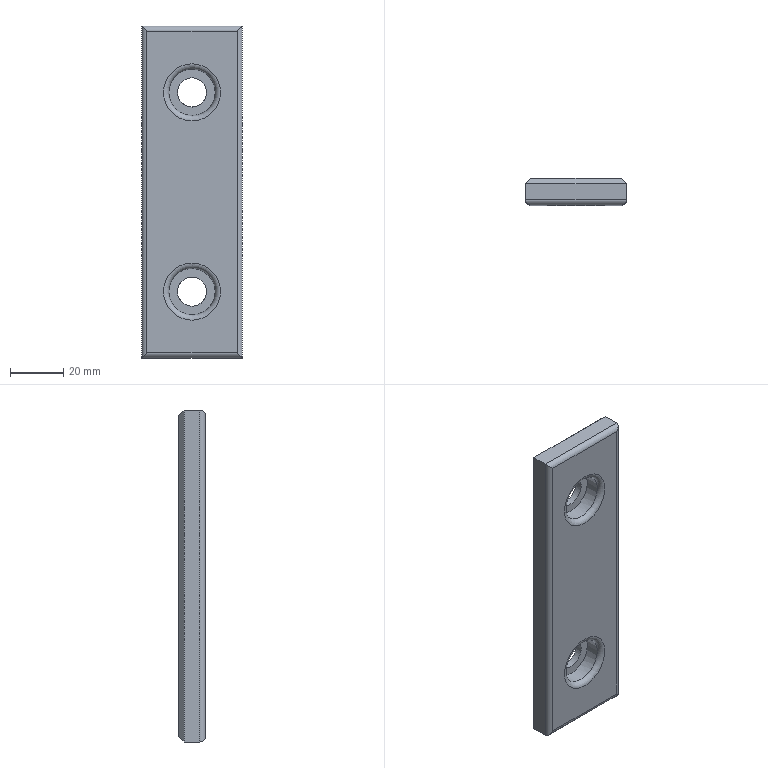Part | NX | features MAIN_BODY 2 | 1 solid | 22 faces | box 38 x 10 x 125 mm | volume 42458 mm3 | plane 12 | cylinder 8 | torus 2 | commonest cylinder face diameters 4 x4 11 x2 17.5 x2
STEP:
#1=CARTESIAN_POINT('',(356.,395.,-133.75));
#2=VERTEX_POINT('',#1);
#3=CARTESIAN_POINT('',(356.,395.,-125.));
#4=DIRECTION('',(0.,-1.,0.));
#5=DIRECTION('',(0.,0.,-1.));
#6=AXIS2_PLACEMENT_3D('',#3,#4,#5);
#7=CIRCLE('',#6,8.75);
#8=EDGE_CURVE('',#2,#2,#7,.T.);
#9=ORIENTED_EDGE('',*,*,#8,.T.);
#10=EDGE_LOOP('',(#9));
#11=FACE_BOUND('',#10,.T.);
#12=CARTESIAN_POINT('',(364.75,400.3,-125.));
#13=VERTEX_POINT('',#12);
#14=CARTESIAN_POINT('',(356.,400.3,-125.));
#15=DIRECTION('',(0.,1.,0.));
#16=DIRECTION('',(1.,0.,0.));
#17=AXIS2_PLACEMENT_3D('',#14,#15,#16);
#18=CIRCLE('',#17,8.75);
#19=EDGE_CURVE('',#13,#13,#18,.T.);
#20=ORIENTED_EDGE('',*,*,#19,.T.);
#21=EDGE_LOOP('',(#20));
#22=FACE_BOUND('',#21,.T.);
#23=CARTESIAN_POINT('',(356.,373.,-125.));
#24=DIRECTION('',(0.,1.,0.));
#25=DIRECTION('',(0.,0.,1.));
#26=AXIS2_PLACEMENT_3D('',#23,#24,#25);
#27=CYLINDRICAL_SURFACE('',#26,8.75);
#28=ADVANCED_FACE('',(#11,#22),#27,.F.);
#29=ORIENTED_EDGE('',*,*,#19,.F.);
#30=EDGE_LOOP('',(#29));
#31=FACE_BOUND('',#30,.T.);
#32=CARTESIAN_POINT('',(356.,400.3,-119.5));
#33=VERTEX_POINT('',#32);
#34=CARTESIAN_POINT('',(356.,400.3,-125.));
#35=DIRECTION('',(0.,1.,0.));
#36=DIRECTION('',(0.,0.,1.));
#37=AXIS2_PLACEMENT_3D('',#34,#35,#36);
#38=CIRCLE('',#37,5.5);
#39=EDGE_CURVE('',#33,#33,#38,.F.);
#40=ORIENTED_EDGE('',*,*,#39,.F.);
#41=EDGE_LOOP('',(#40));
#42=FACE_BOUND('',#41,.T.);
#43=CARTESIAN_POINT('',(356.,400.3,-125.));
#44=DIRECTION('',(0.,1.,0.));
#45=DIRECTION('',(0.,0.,1.));
#46=AXIS2_PLACEMENT_3D('',#43,#44,#45);
#47=PLANE('',#46);
#48=ADVANCED_FACE('',(#31,#42),#47,.F.);
#49=CARTESIAN_POINT('',(356.,393.,-135.75));
#50=VERTEX_POINT('',#49);
#51=CARTESIAN_POINT('',(356.,393.,-125.));
#52=DIRECTION('',(0.,-1.,0.));
#53=DIRECTION('',(0.,0.,-1.));
#54=AXIS2_PLACEMENT_3D('',#51,#52,#53);
#55=CIRCLE('',#54,10.75);
#56=EDGE_CURVE('',#50,#50,#55,.F.);
#57=ORIENTED_EDGE('',*,*,#56,.F.);
#58=EDGE_LOOP('',(#57));
#59=FACE_BOUND('',#58,.T.);
#60=ORIENTED_EDGE('',*,*,#8,.F.);
#61=EDGE_LOOP('',(#60));
#62=FACE_BOUND('',#61,.T.);
#63=CARTESIAN_POINT('',(356.,395.,-125.));
#64=DIRECTION('',(0.,-1.,0.));
#65=DIRECTION('',(0.,0.,-1.));
#66=AXIS2_PLACEMENT_3D('',#63,#64,#65);
#67=TOROIDAL_SURFACE('',#66,10.75,2.);
#68=ADVANCED_FACE('',(#59,#62),#67,.T.);
#69=ORIENTED_EDGE('',*,*,#39,.T.);
#70=EDGE_LOOP('',(#69));
#71=FACE_BOUND('',#70,.T.);
#72=CARTESIAN_POINT('',(361.5,403.,-125.));
#73=VERTEX_POINT('',#72);
#74=CARTESIAN_POINT('',(356.,403.,-125.));
#75=DIRECTION('',(0.,1.,0.));
#76=DIRECTION('',(1.,0.,0.));
#77=AXIS2_PLACEMENT_3D('',#74,#75,#76);
#78=CIRCLE('',#77,5.5);
#79=EDGE_CURVE('',#73,#73,#78,.T.);
#80=ORIENTED_EDGE('',*,*,#79,.T.);
#81=EDGE_LOOP('',(#80));
#82=FACE_BOUND('',#81,.T.);
#83=CARTESIAN_POINT('',(356.,383.,-125.));
#84=DIRECTION('',(0.,1.,0.));
#85=DIRECTION('',(0.,0.,1.));
#86=AXIS2_PLACEMENT_3D('',#83,#84,#85);
#87=CYLINDRICAL_SURFACE('',#86,5.5);
#88=ADVANCED_FACE('',(#71,#82),#87,.F.);
#89=CARTESIAN_POINT('',(375.,395.,-100.));
#90=VERTEX_POINT('',#89);
#91=CARTESIAN_POINT('',(375.,401.,-100.));
#92=VERTEX_POINT('',#91);
#93=CARTESIAN_POINT('',(375.,393.,-100.));
#94=DIRECTION('',(0.,1.,0.));
#95=VECTOR('',#94,1000.);
#96=LINE('',#93,#95);
#97=EDGE_CURVE('',#90,#92,#96,.T.);
#98=ORIENTED_EDGE('',*,*,#97,.T.);
#99=CARTESIAN_POINT('',(337.,401.,-100.));
#100=VERTEX_POINT('',#99);
#101=CARTESIAN_POINT('',(337.,401.,-100.));
#102=DIRECTION('',(-1.,0.,0.));
#103=VECTOR('',#102,1000.);
#104=LINE('',#101,#103);
#105=EDGE_CURVE('',#92,#100,#104,.T.);
#106=ORIENTED_EDGE('',*,*,#105,.T.);
#107=CARTESIAN_POINT('',(337.,395.,-100.));
#108=VERTEX_POINT('',#107);
#109=CARTESIAN_POINT('',(337.,393.,-100.));
#110=DIRECTION('',(0.,1.,0.));
#111=VECTOR('',#110,1000.);
#112=LINE('',#109,#111);
#113=EDGE_CURVE('',#108,#100,#112,.T.);
#114=ORIENTED_EDGE('',*,*,#113,.F.);
#115=CARTESIAN_POINT('',(337.,395.,-100.));
#116=DIRECTION('',(1.,0.,0.));
#117=VECTOR('',#116,1000.);
#118=LINE('',#115,#117);
#119=EDGE_CURVE('',#108,#90,#118,.T.);
#120=ORIENTED_EDGE('',*,*,#119,.T.);
#121=EDGE_LOOP('',(#98,#106,#114,#120));
#122=FACE_BOUND('',#121,.T.);
#123=CARTESIAN_POINT('',(337.,393.,-100.));
#124=DIRECTION('',(0.,0.,1.));
#125=DIRECTION('',(0.,-1.,0.));
#126=AXIS2_PLACEMENT_3D('',#123,#124,#125);
#127=PLANE('',#126);
#128=ADVANCED_FACE('',(#122),#127,.T.);
#129=CARTESIAN_POINT('',(339.,393.,-102.));
#130=VERTEX_POINT('',#129);
#131=CARTESIAN_POINT('',(339.,395.,-102.));
#132=DIRECTION('',(0.7071,0.,0.7071));
#133=DIRECTION('',(0.7071,0.,-0.7071));
#134=AXIS2_PLACEMENT_3D('',#131,#132,#133);
#135=ELLIPSE('',#134,2.828,2.);
#136=EDGE_CURVE('',#130,#108,#135,.F.);
#137=ORIENTED_EDGE('',*,*,#136,.F.);
#138=CARTESIAN_POINT('',(373.,393.,-102.));
#139=VERTEX_POINT('',#138);
#140=CARTESIAN_POINT('',(337.,393.,-102.));
#141=DIRECTION('',(1.,0.,0.));
#142=VECTOR('',#141,1000.);
#143=LINE('',#140,#142);
#144=EDGE_CURVE('',#139,#130,#143,.F.);
#145=ORIENTED_EDGE('',*,*,#144,.F.);
#146=CARTESIAN_POINT('',(373.,395.,-102.));
#147=DIRECTION('',(0.7071,0.,-0.7071));
#148=DIRECTION('',(0.7071,0.,0.7071));
#149=AXIS2_PLACEMENT_3D('',#146,#147,#148);
#150=ELLIPSE('',#149,2.828,2.);
#151=EDGE_CURVE('',#90,#139,#150,.T.);
#152=ORIENTED_EDGE('',*,*,#151,.F.);
#153=ORIENTED_EDGE('',*,*,#119,.F.);
#154=EDGE_LOOP('',(#137,#145,#152,#153));
#155=FACE_BOUND('',#154,.T.);
#156=CARTESIAN_POINT('',(337.,395.,-102.));
#157=DIRECTION('',(1.,0.,0.));
#158=DIRECTION('',(0.,0.,1.));
#159=AXIS2_PLACEMENT_3D('',#156,#157,#158);
#160=CYLINDRICAL_SURFACE('',#159,2.);
#161=ADVANCED_FACE('',(#155),#160,.T.);
#162=CARTESIAN_POINT('',(339.,403.,-102.));
#163=VERTEX_POINT('',#162);
#164=CARTESIAN_POINT('',(338.333,402.333,-101.333));
#165=DIRECTION('',(-0.5774,-0.5774,0.5774));
#166=VECTOR('',#165,1000.);
#167=LINE('',#164,#166);
#168=EDGE_CURVE('',#100,#163,#167,.F.);
#169=ORIENTED_EDGE('',*,*,#168,.F.);
#170=ORIENTED_EDGE('',*,*,#105,.F.);
#171=CARTESIAN_POINT('',(373.,403.,-102.));
#172=VERTEX_POINT('',#171);
#173=CARTESIAN_POINT('',(323.667,452.333,-151.333));
#174=DIRECTION('',(0.5774,-0.5774,0.5774));
#175=VECTOR('',#174,1000.);
#176=LINE('',#173,#175);
#177=EDGE_CURVE('',#172,#92,#176,.T.);
#178=ORIENTED_EDGE('',*,*,#177,.F.);
#179=CARTESIAN_POINT('',(375.,403.,-102.));
#180=DIRECTION('',(1.,0.,0.));
#181=VECTOR('',#180,1000.);
#182=LINE('',#179,#181);
#183=EDGE_CURVE('',#163,#172,#182,.T.);
#184=ORIENTED_EDGE('',*,*,#183,.F.);
#185=EDGE_LOOP('',(#169,#170,#178,#184));
#186=FACE_BOUND('',#185,.T.);
#187=CARTESIAN_POINT('',(337.,403.,-102.));
#188=DIRECTION('',(0.,0.7071,0.7071));
#189=DIRECTION('',(0.,-0.7071,0.7071));
#190=AXIS2_PLACEMENT_3D('',#187,#188,#189);
#191=PLANE('',#190);
#192=ADVANCED_FACE('',(#186),#191,.T.);
#193=CARTESIAN_POINT('',(373.,403.,-223.));
#194=VERTEX_POINT('',#193);
#195=CARTESIAN_POINT('',(375.,401.,-225.));
#196=VERTEX_POINT('',#195);
#197=CARTESIAN_POINT('',(373.667,402.333,-223.667));
#198=DIRECTION('',(-0.5774,0.5774,0.5774));
#199=VECTOR('',#198,1000.);
#200=LINE('',#197,#199);
#201=EDGE_CURVE('',#194,#196,#200,.F.);
#202=ORIENTED_EDGE('',*,*,#201,.F.);
#203=CARTESIAN_POINT('',(373.,403.,-250.));
#204=DIRECTION('',(0.,0.,-1.));
#205=VECTOR('',#204,1000.);
#206=LINE('',#203,#205);
#207=EDGE_CURVE('',#172,#194,#206,.T.);
#208=ORIENTED_EDGE('',*,*,#207,.F.);
#209=ORIENTED_EDGE('',*,*,#177,.T.);
#210=CARTESIAN_POINT('',(375.,401.,-100.));
#211=DIRECTION('',(0.,0.,1.));
#212=VECTOR('',#211,1000.);
#213=LINE('',#210,#212);
#214=EDGE_CURVE('',#196,#92,#213,.T.);
#215=ORIENTED_EDGE('',*,*,#214,.F.);
#216=EDGE_LOOP('',(#202,#208,#209,#215));
#217=FACE_BOUND('',#216,.T.);
#218=CARTESIAN_POINT('',(373.,403.,-250.));
#219=DIRECTION('',(0.7071,0.7071,0.));
#220=DIRECTION('',(-0.7071,0.7071,0.));
#221=AXIS2_PLACEMENT_3D('',#218,#219,#220);
#222=PLANE('',#221);
#223=ADVANCED_FACE('',(#217),#222,.T.);
#224=CARTESIAN_POINT('',(375.,395.,-225.));
#225=VERTEX_POINT('',#224);
#226=CARTESIAN_POINT('',(373.,393.,-223.));
#227=VERTEX_POINT('',#226);
#228=CARTESIAN_POINT('',(373.,395.,-223.));
#229=DIRECTION('',(-0.7071,0.,-0.7071));
#230=DIRECTION('',(0.7071,0.,-0.7071));
#231=AXIS2_PLACEMENT_3D('',#228,#229,#230);
#232=ELLIPSE('',#231,2.828,2.);
#233=EDGE_CURVE('',#225,#227,#232,.T.);
#234=ORIENTED_EDGE('',*,*,#233,.F.);
#235=CARTESIAN_POINT('',(375.,395.,-100.));
#236=DIRECTION('',(0.,0.,-1.));
#237=VECTOR('',#236,1000.);
#238=LINE('',#235,#237);
#239=EDGE_CURVE('',#90,#225,#238,.T.);
#240=ORIENTED_EDGE('',*,*,#239,.F.);
#241=ORIENTED_EDGE('',*,*,#151,.T.);
#242=CARTESIAN_POINT('',(373.,393.,-250.));
#243=DIRECTION('',(0.,0.,-1.));
#244=VECTOR('',#243,1000.);
#245=LINE('',#242,#244);
#246=EDGE_CURVE('',#227,#139,#245,.F.);
#247=ORIENTED_EDGE('',*,*,#246,.F.);
#248=EDGE_LOOP('',(#234,#240,#241,#247));
#249=FACE_BOUND('',#248,.T.);
#250=CARTESIAN_POINT('',(373.,395.,-100.));
#251=DIRECTION('',(0.,0.,-1.));
#252=DIRECTION('',(0.,1.,0.));
#253=AXIS2_PLACEMENT_3D('',#250,#251,#252);
#254=CYLINDRICAL_SURFACE('',#253,2.);
#255=ADVANCED_FACE('',(#249),#254,.T.);
#256=ORIENTED_EDGE('',*,*,#214,.T.);
#257=ORIENTED_EDGE('',*,*,#97,.F.);
#258=ORIENTED_EDGE('',*,*,#239,.T.);
#259=CARTESIAN_POINT('',(375.,393.,-225.));
#260=DIRECTION('',(0.,1.,0.));
#261=VECTOR('',#260,1000.);
#262=LINE('',#259,#261);
#263=EDGE_CURVE('',#225,#196,#262,.T.);
#264=ORIENTED_EDGE('',*,*,#263,.T.);
#265=EDGE_LOOP('',(#256,#257,#258,#264));
#266=FACE_BOUND('',#265,.T.);
#267=CARTESIAN_POINT('',(375.,393.,-100.));
#268=DIRECTION('',(1.,0.,0.));
#269=DIRECTION('',(0.,0.,1.));
#270=AXIS2_PLACEMENT_3D('',#267,#268,#269);
#271=PLANE('',#270);
#272=ADVANCED_FACE('',(#266),#271,.T.);
#273=CARTESIAN_POINT('',(339.,393.,-223.));
#274=VERTEX_POINT('',#273);
#275=CARTESIAN_POINT('',(337.,395.,-225.));
#276=VERTEX_POINT('',#275);
#277=CARTESIAN_POINT('',(339.,395.,-223.));
#278=DIRECTION('',(-0.7071,0.,0.7071));
#279=DIRECTION('',(0.7071,0.,0.7071));
#280=AXIS2_PLACEMENT_3D('',#277,#278,#279);
#281=ELLIPSE('',#280,2.828,2.);
#282=EDGE_CURVE('',#274,#276,#281,.F.);
#283=ORIENTED_EDGE('',*,*,#282,.F.);
#284=CARTESIAN_POINT('',(339.,393.,-250.));
#285=DIRECTION('',(0.,0.,1.));
#286=VECTOR('',#285,1000.);
#287=LINE('',#284,#286);
#288=EDGE_CURVE('',#130,#274,#287,.F.);
#289=ORIENTED_EDGE('',*,*,#288,.F.);
#290=ORIENTED_EDGE('',*,*,#136,.T.);
#291=CARTESIAN_POINT('',(337.,395.,-250.));
#292=DIRECTION('',(0.,0.,1.));
#293=VECTOR('',#292,1000.);
#294=LINE('',#291,#293);
#295=EDGE_CURVE('',#276,#108,#294,.T.);
#296=ORIENTED_EDGE('',*,*,#295,.F.);
#297=EDGE_LOOP('',(#283,#289,#290,#296));
#298=FACE_BOUND('',#297,.T.);
#299=CARTESIAN_POINT('',(339.,395.,-250.));
#300=DIRECTION('',(0.,0.,1.));
#301=DIRECTION('',(-1.,0.,0.));
#302=AXIS2_PLACEMENT_3D('',#299,#300,#301);
#303=CYLINDRICAL_SURFACE('',#302,2.);
#304=ADVANCED_FACE('',(#298),#303,.T.);
#305=CARTESIAN_POINT('',(337.,401.,-225.));
#306=VERTEX_POINT('',#305);
#307=CARTESIAN_POINT('',(339.,403.,-223.));
#308=VERTEX_POINT('',#307);
#309=CARTESIAN_POINT('',(338.333,402.333,-223.667));
#310=DIRECTION('',(-0.5774,-0.5774,-0.5774));
#311=VECTOR('',#310,1000.);
#312=LINE('',#309,#311);
#313=EDGE_CURVE('',#306,#308,#312,.F.);
#314=ORIENTED_EDGE('',*,*,#313,.F.);
#315=CARTESIAN_POINT('',(337.,401.,-250.));
#316=DIRECTION('',(0.,0.,-1.));
#317=VECTOR('',#316,1000.);
#318=LINE('',#315,#317);
#319=EDGE_CURVE('',#100,#306,#318,.T.);
#320=ORIENTED_EDGE('',*,*,#319,.F.);
#321=ORIENTED_EDGE('',*,*,#168,.T.);
#322=CARTESIAN_POINT('',(339.,403.,-100.));
#323=DIRECTION('',(0.,0.,1.));
#324=VECTOR('',#323,1000.);
#325=LINE('',#322,#324);
#326=EDGE_CURVE('',#308,#163,#325,.T.);
#327=ORIENTED_EDGE('',*,*,#326,.F.);
#328=EDGE_LOOP('',(#314,#320,#321,#327));
#329=FACE_BOUND('',#328,.T.);
#330=CARTESIAN_POINT('',(339.,403.,-250.));
#331=DIRECTION('',(-0.7071,0.7071,0.));
#332=DIRECTION('',(-0.7071,-0.7071,0.));
#333=AXIS2_PLACEMENT_3D('',#330,#331,#332);
#334=PLANE('',#333);
#335=ADVANCED_FACE('',(#329),#334,.T.);
#336=ORIENTED_EDGE('',*,*,#295,.T.);
#337=ORIENTED_EDGE('',*,*,#113,.T.);
#338=ORIENTED_EDGE('',*,*,#319,.T.);
#339=CARTESIAN_POINT('',(337.,393.,-225.));
#340=DIRECTION('',(0.,1.,0.));
#341=VECTOR('',#340,1000.);
#342=LINE('',#339,#341);
#343=EDGE_CURVE('',#276,#306,#342,.T.);
#344=ORIENTED_EDGE('',*,*,#343,.F.);
#345=EDGE_LOOP('',(#336,#337,#338,#344));
#346=FACE_BOUND('',#345,.T.);
#347=CARTESIAN_POINT('',(337.,393.,-250.));
#348=DIRECTION('',(-1.,0.,0.));
#349=DIRECTION('',(0.,0.,-1.));
#350=AXIS2_PLACEMENT_3D('',#347,#348,#349);
#351=PLANE('',#350);
#352=ADVANCED_FACE('',(#346),#351,.T.);
#353=ORIENTED_EDGE('',*,*,#326,.T.);
#354=ORIENTED_EDGE('',*,*,#183,.T.);
#355=ORIENTED_EDGE('',*,*,#207,.T.);
#356=CARTESIAN_POINT('',(337.,403.,-223.));
#357=DIRECTION('',(-1.,0.,0.));
#358=VECTOR('',#357,1000.);
#359=LINE('',#356,#358);
#360=EDGE_CURVE('',#194,#308,#359,.T.);
#361=ORIENTED_EDGE('',*,*,#360,.T.);
#362=EDGE_LOOP('',(#353,#354,#355,#361));
#363=FACE_BOUND('',#362,.T.);
#364=ORIENTED_EDGE('',*,*,#79,.F.);
#365=EDGE_LOOP('',(#364));
#366=FACE_BOUND('',#365,.T.);
#367=CARTESIAN_POINT('',(361.5,403.,-200.));
#368=VERTEX_POINT('',#367);
#369=CARTESIAN_POINT('',(356.,403.,-200.));
#370=DIRECTION('',(0.,-1.,0.));
#371=DIRECTION('',(1.,0.,0.));
#372=AXIS2_PLACEMENT_3D('',#369,#370,#371);
#373=CIRCLE('',#372,5.5);
#374=EDGE_CURVE('',#368,#368,#373,.T.);
#375=ORIENTED_EDGE('',*,*,#374,.T.);
#376=EDGE_LOOP('',(#375));
#377=FACE_BOUND('',#376,.T.);
#378=CARTESIAN_POINT('',(337.,403.,-250.));
#379=DIRECTION('',(0.,-1.,0.));
#380=DIRECTION('',(0.,0.,-1.));
#381=AXIS2_PLACEMENT_3D('',#378,#379,#380);
#382=PLANE('',#381);
#383=ADVANCED_FACE('',(#363,#366,#377),#382,.F.);
#384=ORIENTED_EDGE('',*,*,#246,.T.);
#385=ORIENTED_EDGE('',*,*,#144,.T.);
#386=ORIENTED_EDGE('',*,*,#288,.T.);
#387=CARTESIAN_POINT('',(337.,393.,-223.));
#388=DIRECTION('',(-1.,0.,0.));
#389=VECTOR('',#388,1000.);
#390=LINE('',#387,#389);
#391=EDGE_CURVE('',#274,#227,#390,.F.);
#392=ORIENTED_EDGE('',*,*,#391,.T.);
#393=EDGE_LOOP('',(#384,#385,#386,#392));
#394=FACE_BOUND('',#393,.T.);
#395=ORIENTED_EDGE('',*,*,#56,.T.);
#396=EDGE_LOOP('',(#395));
#397=FACE_BOUND('',#396,.T.);
#398=CARTESIAN_POINT('',(356.,393.,-210.75));
#399=VERTEX_POINT('',#398);
#400=CARTESIAN_POINT('',(356.,393.,-200.));
#401=DIRECTION('',(0.,-1.,0.));
#402=DIRECTION('',(0.,0.,-1.));
#403=AXIS2_PLACEMENT_3D('',#400,#401,#402);
#404=CIRCLE('',#403,10.75);
#405=EDGE_CURVE('',#399,#399,#404,.F.);
#406=ORIENTED_EDGE('',*,*,#405,.T.);
#407=EDGE_LOOP('',(#406));
#408=FACE_BOUND('',#407,.T.);
#409=CARTESIAN_POINT('',(337.,393.,-250.));
#410=DIRECTION('',(0.,-1.,0.));
#411=DIRECTION('',(0.,0.,-1.));
#412=AXIS2_PLACEMENT_3D('',#409,#410,#411);
#413=PLANE('',#412);
#414=ADVANCED_FACE('',(#394,#397,#408),#413,.T.);
#415=ORIENTED_EDGE('',*,*,#374,.F.);
#416=EDGE_LOOP('',(#415));
#417=FACE_BOUND('',#416,.T.);
#418=CARTESIAN_POINT('',(356.,400.3,-205.5));
#419=VERTEX_POINT('',#418);
#420=CARTESIAN_POINT('',(356.,400.3,-200.));
#421=DIRECTION('',(0.,-1.,0.));
#422=DIRECTION('',(0.,0.,-1.));
#423=AXIS2_PLACEMENT_3D('',#420,#421,#422);
#424=CIRCLE('',#423,5.5);
#425=EDGE_CURVE('',#419,#419,#424,.T.);
#426=ORIENTED_EDGE('',*,*,#425,.T.);
#427=EDGE_LOOP('',(#426));
#428=FACE_BOUND('',#427,.T.);
#429=CARTESIAN_POINT('',(356.,383.,-200.));
#430=DIRECTION('',(0.,1.,0.));
#431=DIRECTION('',(0.,0.,1.));
#432=AXIS2_PLACEMENT_3D('',#429,#430,#431);
#433=CYLINDRICAL_SURFACE('',#432,5.5);
#434=ADVANCED_FACE('',(#417,#428),#433,.F.);
#435=ORIENTED_EDGE('',*,*,#343,.T.);
#436=CARTESIAN_POINT('',(375.,401.,-225.));
#437=DIRECTION('',(1.,0.,0.));
#438=VECTOR('',#437,1000.);
#439=LINE('',#436,#438);
#440=EDGE_CURVE('',#306,#196,#439,.T.);
#441=ORIENTED_EDGE('',*,*,#440,.T.);
#442=ORIENTED_EDGE('',*,*,#263,.F.);
#443=CARTESIAN_POINT('',(375.,395.,-225.));
#444=DIRECTION('',(-1.,0.,0.));
#445=VECTOR('',#444,1000.);
#446=LINE('',#443,#445);
#447=EDGE_CURVE('',#225,#276,#446,.T.);
#448=ORIENTED_EDGE('',*,*,#447,.T.);
#449=EDGE_LOOP('',(#435,#441,#442,#448));
#450=FACE_BOUND('',#449,.T.);
#451=CARTESIAN_POINT('',(375.,393.,-225.));
#452=DIRECTION('',(0.,0.,-1.));
#453=DIRECTION('',(1.,0.,0.));
#454=AXIS2_PLACEMENT_3D('',#451,#452,#453);
#455=PLANE('',#454);
#456=ADVANCED_FACE('',(#450),#455,.T.);
#457=CARTESIAN_POINT('',(356.,395.,-208.75));
#458=VERTEX_POINT('',#457);
#459=CARTESIAN_POINT('',(356.,395.,-200.));
#460=DIRECTION('',(0.,-1.,0.));
#461=DIRECTION('',(0.,0.,-1.));
#462=AXIS2_PLACEMENT_3D('',#459,#460,#461);
#463=CIRCLE('',#462,8.75);
#464=EDGE_CURVE('',#458,#458,#463,.T.);
#465=ORIENTED_EDGE('',*,*,#464,.T.);
#466=EDGE_LOOP('',(#465));
#467=FACE_BOUND('',#466,.T.);
#468=CARTESIAN_POINT('',(364.75,400.3,-200.));
#469=VERTEX_POINT('',#468);
#470=CARTESIAN_POINT('',(356.,400.3,-200.));
#471=DIRECTION('',(0.,-1.,0.));
#472=DIRECTION('',(1.,0.,0.));
#473=AXIS2_PLACEMENT_3D('',#470,#471,#472);
#474=CIRCLE('',#473,8.75);
#475=EDGE_CURVE('',#469,#469,#474,.T.);
#476=ORIENTED_EDGE('',*,*,#475,.F.);
#477=EDGE_LOOP('',(#476));
#478=FACE_BOUND('',#477,.T.);
#479=CARTESIAN_POINT('',(356.,373.,-200.));
#480=DIRECTION('',(0.,1.,0.));
#481=DIRECTION('',(0.,0.,1.));
#482=AXIS2_PLACEMENT_3D('',#479,#480,#481);
#483=CYLINDRICAL_SURFACE('',#482,8.75);
#484=ADVANCED_FACE('',(#467,#478),#483,.F.);
#485=ORIENTED_EDGE('',*,*,#425,.F.);
#486=EDGE_LOOP('',(#485));
#487=FACE_BOUND('',#486,.T.);
#488=ORIENTED_EDGE('',*,*,#475,.T.);
#489=EDGE_LOOP('',(#488));
#490=FACE_BOUND('',#489,.T.);
#491=CARTESIAN_POINT('',(356.,400.3,-200.));
#492=DIRECTION('',(0.,-1.,0.));
#493=DIRECTION('',(0.,0.,-1.));
#494=AXIS2_PLACEMENT_3D('',#491,#492,#493);
#495=PLANE('',#494);
#496=ADVANCED_FACE('',(#487,#490),#495,.T.);
#497=ORIENTED_EDGE('',*,*,#233,.T.);
#498=ORIENTED_EDGE('',*,*,#391,.F.);
#499=ORIENTED_EDGE('',*,*,#282,.T.);
#500=ORIENTED_EDGE('',*,*,#447,.F.);
#501=EDGE_LOOP('',(#497,#498,#499,#500));
#502=FACE_BOUND('',#501,.T.);
#503=CARTESIAN_POINT('',(375.,395.,-223.));
#504=DIRECTION('',(-1.,0.,0.));
#505=DIRECTION('',(0.,0.,-1.));
#506=AXIS2_PLACEMENT_3D('',#503,#504,#505);
#507=CYLINDRICAL_SURFACE('',#506,2.);
#508=ADVANCED_FACE('',(#502),#507,.T.);
#509=ORIENTED_EDGE('',*,*,#464,.F.);
#510=EDGE_LOOP('',(#509));
#511=FACE_BOUND('',#510,.T.);
#512=ORIENTED_EDGE('',*,*,#405,.F.);
#513=EDGE_LOOP('',(#512));
#514=FACE_BOUND('',#513,.T.);
#515=CARTESIAN_POINT('',(356.,395.,-200.));
#516=DIRECTION('',(0.,-1.,0.));
#517=DIRECTION('',(0.,0.,-1.));
#518=AXIS2_PLACEMENT_3D('',#515,#516,#517);
#519=TOROIDAL_SURFACE('',#518,10.75,2.);
#520=ADVANCED_FACE('',(#511,#514),#519,.T.);
#521=ORIENTED_EDGE('',*,*,#201,.T.);
#522=ORIENTED_EDGE('',*,*,#440,.F.);
#523=ORIENTED_EDGE('',*,*,#313,.T.);
#524=ORIENTED_EDGE('',*,*,#360,.F.);
#525=EDGE_LOOP('',(#521,#522,#523,#524));
#526=FACE_BOUND('',#525,.T.);
#527=CARTESIAN_POINT('',(337.,403.,-223.));
#528=DIRECTION('',(0.,0.7071,-0.7071));
#529=DIRECTION('',(0.,0.7071,0.7071));
#530=AXIS2_PLACEMENT_3D('',#527,#528,#529);
#531=PLANE('',#530);
#532=ADVANCED_FACE('',(#526),#531,.T.);
#533=CLOSED_SHELL('',(#28,#48,#68,#88,#128,#161,#192,#223,#255,#272,#304,#335,#352,#383,#414,#434,#456,#484,#496,#508,#520,#532));
#534=MANIFOLD_SOLID_BREP('',#533);
#535=(LENGTH_UNIT()NAMED_UNIT(*)SI_UNIT(.MILLI.,.METRE.));
#536=UNCERTAINTY_MEASURE_WITH_UNIT(LENGTH_MEASURE(0.00001),#535,'','');
#537=(NAMED_UNIT(*)PLANE_ANGLE_UNIT()SI_UNIT($,.RADIAN.));
#538=(NAMED_UNIT(*)SI_UNIT($,.STERADIAN.)SOLID_ANGLE_UNIT());
#539=(GEOMETRIC_REPRESENTATION_CONTEXT(3)GLOBAL_UNCERTAINTY_ASSIGNED_CONTEXT((#536))GLOBAL_UNIT_ASSIGNED_CONTEXT((#535,#537,#538))REPRESENTATION_CONTEXT('',''));
#540=ADVANCED_BREP_SHAPE_REPRESENTATION('',(#534),#539);